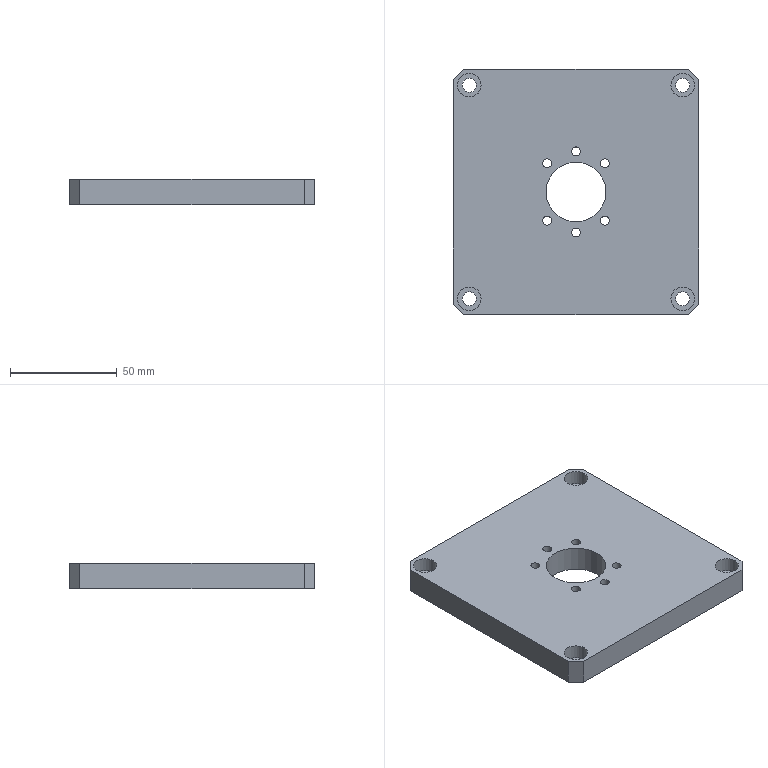CAM job | NX | 3-axis milling, drilling | part box 115 x 115 x 12 mm | stock box 120 x 120 x 15 mm
Tools:
number,name,description,diameter,corner_radius,flute_length,length,flutes
6,D6,平底铣刀-粗,6.0,0.0,25.0,75.0,2
9,D10,平底铣刀-粗,10.0,0.0,35.0,75.0,2
7,D6-J,平底铣刀-精,6.0,0.0,25.0,75.0,2
10,D10-J,平底铣刀-精,10.0,0.0,35.0,75.0,2
1,D80R0.8飞刀,圆鼻刀-粗,80.0,0.8,50.0,75.0,2
1,D80R0.8飞刀-J,圆鼻刀-精,80.0,0.8,50.0,75.0,2
2,D6倒角刀,倒角刀,6.0,0.0,3.0,25.0,2
22,M5X0.8,丝锥,4.2,0.0,35.0,50.0,2
17,ZT6.6,钻头,6.6,0.0,35.0,50.0,2
18,ZT12,钻头,12.0,0.0,35.0,50.0,2
14,钻头4.2,Twist Drill 4.2 mm,4.2,0.0,41.0,41.738,2
Operations:
program,operation,operation_type,tool,method,geometry_group,spindle_rpm,surface_speed,feed_per_tooth,feed_cut,feed_plunge,cut_length_mm,path_length_mm,cut_time_min,machine_time_min
B,底壁铣飞面开粗_COPY,VolumeBased25DMillingOperation,D80R0.8飞刀,分层开粗-切深K-步距G,W-B,2800.0,703.696,0.5357,3000.0,100.0,2828.125,3160.685,0.9427,0.976
B,底壁铣飞面精光_COPY,VolumeBased25DMillingOperation,D80R0.8飞刀-J,侧刃精光-切深K-步距G,W-B,4000.0,1005.28,0.125,1000.0,100.0,470.767,506.767,0.4708,0.4744
B,钻倒角_1,Operation,D6倒角刀,METHOD,W-B,8000.0,150.796,0.0625,1000.0,0.0,34.2,209.83,0.0342,0.0518
B,铣倒角_4,PlanarMilling,D6倒角刀,METHOD,W-B,8000.0,150.796,0.075,1200.0,100.0,81.784,549.008,0.0682,0.1149
B,C0.3封闭铣廓倒角6X45L_COPY,PlanarMilling,D6倒角刀,爬面_倒角-切深0-步距G,W-B,7000.0,131.0,0.1071,1500.0,100.0,562.612,699.851,0.3751,0.3888
A,顶面,FaceMilling,D80R0.8飞刀,侧刃精光-切深K-步距G,W-A,4000.0,1005.31,0.125,1000.0,100.0,696.5,732.5,0.6965,0.7001
A,外形粗_2,VolumeBased25DMillingOperation,D10,METHOD,W-A,8000.0,251.327,0.3125,5000.0,80.0,8167.095,8217.795,1.633,1.639
A,打点0.8,Operation,D6倒角刀,METHOD,W-A,8000.0,150.796,0.0312,500.0,0.0,1.8,43.6,0.0036,0.0078
A,打点-深0.8,Operation,D6倒角刀,NONE,W-A,8000.0,150.796,0.0312,500.0,90.0,18.0,450.192,0.036,0.0792
A,通孔-M5螺纹底孔,Operation,钻头4.2,NONE,W-A,3000.0,39.584,0.0583,350.0,90.0,121.571,373.336,0.3473,0.3725
A,沉头孔-钻孔0段,Operation,ZT6.6,NONE,W-A,1200.0,24.881,0.0625,150.0,90.0,67.931,478.878,0.4529,0.494
A,通孔-10-12.5,Operation,ZT12,NONE,W-A,800.0,30.159,0.0938,150.0,90.0,18.605,77.21,0.124,0.1299
A,底壁铣螺旋开粗-中_COPY,VolumeBased25DMillingOperation,D10,分层开粗-切深K-步距G,W-A,8000.0,251.327,0.125,2000.0,100.0,1257.733,1308.233,0.6289,0.6339
A,铣孔开粗D6_1,CylinderMilling,D6,NONE,W-A,8000.0,150.796,0.075,1200.0,100.0,971.613,1456.813,0.8097,0.8582
A,铣孔精光D6_1,CylinderMilling,D6-J,精光步距切深关,W-A,8000.0,150.796,0.0312,500.0,100.0,183.736,670.936,0.3675,0.4162
A,仅选体,SurfaceContour,D6倒角刀,METHOD,W-A,8000.0,150.796,0.1875,3000.0,100.0,554.573,697.643,0.1849,0.1992
A,铣倒角_1,PlanarMilling,D6倒角刀,METHOD,W-A,8000.0,150.796,0.0312,500.0,100.0,108.122,440.774,0.2162,0.2495
A,铣倒角_2,PlanarMilling,D6倒角刀,NONE,W-A,8000.0,150.796,0.05,800.0,100.0,173.57,611.374,0.217,0.2607
A,铣倒角_3,PlanarMilling,D6倒角刀,METHOD,W-A,8000.0,150.796,0.05,800.0,100.0,93.991,134.991,0.1175,0.1216
A,通孔-攻牙M5,Operation,M5X0.8,METHOD,W-A,500.0,6.597,0.0008,0.8,90.0,99.0,328.194,123.75,123.773
A,底壁铣精光侧面-中_COPY,VolumeBased25DMillingOperation,D6-J,侧刃精光-切深K-步距G,W-A,6000.0,113.097,0.0667,800.0,100.0,151.834,194.005,0.1898,0.194
A,外形半精_2,VolumeBased25DMillingOperation,D10-J,METHOD,W-A,8000.0,251.327,0.0625,1000.0,100.0,484.658,548.058,0.4847,0.491